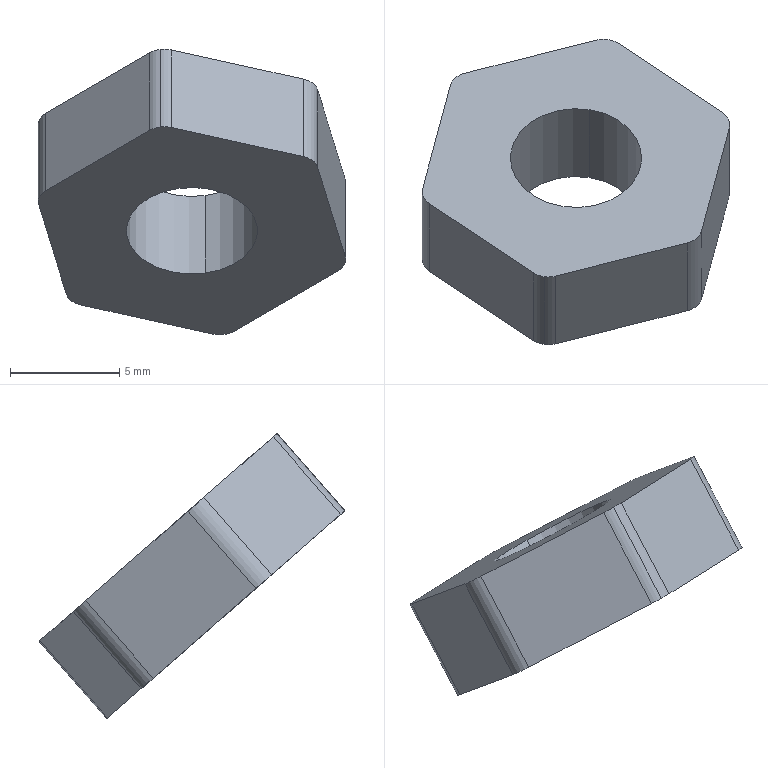Part | STEP file | Fillet 1-12 | 1 solid | 18 faces | box 14.041 x 13.974 x 13.045 mm | volume 553.479 mm3 | cylinder 10 | plane 8 | commonest cylinder face diameters 2 x8 6 x2
STEP:
#1=CARTESIAN_POINT('',(289.281,-940.08,2894.843));
#2=VERTEX_POINT('',#1);
#3=CARTESIAN_POINT('',(288.818,-939.907,2894.691));
#4=VERTEX_POINT('',#3);
#5=CARTESIAN_POINT('',(289.48,-939.342,2894.198));
#6=DIRECTION('',(0.,-0.6579,-0.7531));
#7=DIRECTION('',(0.1984,0.7382,-0.6448));
#8=AXIS2_PLACEMENT_3D('',#5,#6,#7);
#9=CIRCLE('',#8,1.);
#10=EDGE_CURVE('',#2,#4,#9,.T.);
#11=ORIENTED_EDGE('',*,*,#10,.F.);
#12=CARTESIAN_POINT('',(289.281,-936.988,2898.383));
#13=VERTEX_POINT('',#12);
#14=CARTESIAN_POINT('',(289.281,-940.08,2894.843));
#15=DIRECTION('',(0.,0.6579,0.7531));
#16=VECTOR('',#15,1000.);
#17=LINE('',#14,#16);
#18=EDGE_CURVE('',#2,#13,#17,.T.);
#19=ORIENTED_EDGE('',*,*,#18,.T.);
#20=CARTESIAN_POINT('',(288.818,-936.815,2898.231));
#21=VERTEX_POINT('',#20);
#22=CARTESIAN_POINT('',(289.48,-936.25,2897.738));
#23=DIRECTION('',(0.,0.6579,0.7531));
#24=DIRECTION('',(0.1984,0.7382,-0.6448));
#25=AXIS2_PLACEMENT_3D('',#22,#23,#24);
#26=CIRCLE('',#25,1.);
#27=EDGE_CURVE('',#21,#13,#26,.T.);
#28=ORIENTED_EDGE('',*,*,#27,.F.);
#29=CARTESIAN_POINT('',(288.818,-939.907,2894.691));
#30=DIRECTION('',(0.,0.6579,0.7531));
#31=VECTOR('',#30,1000.);
#32=LINE('',#29,#31);
#33=EDGE_CURVE('',#4,#21,#32,.T.);
#34=ORIENTED_EDGE('',*,*,#33,.F.);
#35=EDGE_LOOP('',(#11,#19,#28,#34));
#36=FACE_OUTER_BOUND('',#35,.T.);
#37=CARTESIAN_POINT('',(289.48,-939.342,2894.198));
#38=DIRECTION('',(0.,0.6579,0.7531));
#39=DIRECTION('',(-0.1984,-0.7382,0.6448));
#40=AXIS2_PLACEMENT_3D('',#37,#38,#39);
#41=CYLINDRICAL_SURFACE('',#40,1.);
#42=ADVANCED_FACE('',(#36),#41,.T.);
#43=CARTESIAN_POINT('',(292.198,-929.228,2885.364));
#44=VERTEX_POINT('',#43);
#45=CARTESIAN_POINT('',(292.661,-929.402,2885.515));
#46=VERTEX_POINT('',#45);
#47=CARTESIAN_POINT('',(292.,-929.966,2886.008));
#48=DIRECTION('',(0.,-0.6579,-0.7531));
#49=DIRECTION('',(0.1984,0.7382,-0.6448));
#50=AXIS2_PLACEMENT_3D('',#47,#48,#49);
#51=CIRCLE('',#50,1.);
#52=EDGE_CURVE('',#44,#46,#51,.T.);
#53=ORIENTED_EDGE('',*,*,#52,.F.);
#54=CARTESIAN_POINT('',(292.198,-926.136,2888.903));
#55=VERTEX_POINT('',#54);
#56=CARTESIAN_POINT('',(292.198,-929.228,2885.364));
#57=DIRECTION('',(0.,0.6579,0.7531));
#58=VECTOR('',#57,1000.);
#59=LINE('',#56,#58);
#60=EDGE_CURVE('',#44,#55,#59,.T.);
#61=ORIENTED_EDGE('',*,*,#60,.T.);
#62=CARTESIAN_POINT('',(292.661,-926.31,2889.055));
#63=VERTEX_POINT('',#62);
#64=CARTESIAN_POINT('',(292.,-926.874,2889.548));
#65=DIRECTION('',(0.,0.6579,0.7531));
#66=DIRECTION('',(0.1984,0.7382,-0.6448));
#67=AXIS2_PLACEMENT_3D('',#64,#65,#66);
#68=CIRCLE('',#67,1.);
#69=EDGE_CURVE('',#63,#55,#68,.T.);
#70=ORIENTED_EDGE('',*,*,#69,.F.);
#71=CARTESIAN_POINT('',(292.661,-929.402,2885.515));
#72=DIRECTION('',(0.,0.6579,0.7531));
#73=VECTOR('',#72,1000.);
#74=LINE('',#71,#73);
#75=EDGE_CURVE('',#46,#63,#74,.T.);
#76=ORIENTED_EDGE('',*,*,#75,.F.);
#77=EDGE_LOOP('',(#53,#61,#70,#76));
#78=FACE_OUTER_BOUND('',#77,.T.);
#79=CARTESIAN_POINT('',(292.,-929.966,2886.008));
#80=DIRECTION('',(0.,0.6579,0.7531));
#81=DIRECTION('',(-0.1984,-0.7382,0.6448));
#82=AXIS2_PLACEMENT_3D('',#79,#80,#81);
#83=CYLINDRICAL_SURFACE('',#82,1.);
#84=ADVANCED_FACE('',(#78),#83,.T.);
#85=CARTESIAN_POINT('',(290.144,-936.869,2892.038));
#86=VERTEX_POINT('',#85);
#87=CARTESIAN_POINT('',(291.335,-932.44,2888.169));
#88=VERTEX_POINT('',#87);
#89=CARTESIAN_POINT('',(290.74,-934.654,2890.103));
#90=DIRECTION('',(0.,0.6579,0.7531));
#91=DIRECTION('',(0.1984,0.7382,-0.6448));
#92=AXIS2_PLACEMENT_3D('',#89,#90,#91);
#93=CIRCLE('',#92,3.);
#94=EDGE_CURVE('',#86,#88,#93,.T.);
#95=ORIENTED_EDGE('',*,*,#94,.F.);
#96=CARTESIAN_POINT('',(290.144,-933.777,2895.578));
#97=VERTEX_POINT('',#96);
#98=CARTESIAN_POINT('',(290.144,-938.711,2889.929));
#99=DIRECTION('',(0.,0.6579,0.7531));
#100=VECTOR('',#99,1000.);
#101=LINE('',#98,#100);
#102=EDGE_CURVE('',#86,#97,#101,.T.);
#103=ORIENTED_EDGE('',*,*,#102,.T.);
#104=CARTESIAN_POINT('',(291.335,-929.348,2891.709));
#105=VERTEX_POINT('',#104);
#106=CARTESIAN_POINT('',(290.74,-931.562,2893.643));
#107=DIRECTION('',(0.,0.6579,0.7531));
#108=DIRECTION('',(0.1984,0.7382,-0.6448));
#109=AXIS2_PLACEMENT_3D('',#106,#107,#108);
#110=CIRCLE('',#109,3.);
#111=EDGE_CURVE('',#97,#105,#110,.T.);
#112=ORIENTED_EDGE('',*,*,#111,.T.);
#113=CARTESIAN_POINT('',(291.335,-934.282,2886.06));
#114=DIRECTION('',(0.,0.6579,0.7531));
#115=VECTOR('',#114,1000.);
#116=LINE('',#113,#115);
#117=EDGE_CURVE('',#88,#105,#116,.T.);
#118=ORIENTED_EDGE('',*,*,#117,.F.);
#119=EDGE_LOOP('',(#95,#103,#112,#118));
#120=FACE_OUTER_BOUND('',#119,.T.);
#121=CARTESIAN_POINT('',(290.74,-936.496,2887.995));
#122=DIRECTION('',(0.,0.6579,0.7531));
#123=DIRECTION('',(-0.1984,-0.7382,0.6448));
#124=AXIS2_PLACEMENT_3D('',#121,#122,#123);
#125=CYLINDRICAL_SURFACE('',#124,3.);
#126=ADVANCED_FACE('',(#120),#125,.F.);
#127=CARTESIAN_POINT('',(297.422,-932.568,2888.281));
#128=VERTEX_POINT('',#127);
#129=CARTESIAN_POINT('',(297.855,-932.855,2888.532));
#130=DIRECTION('',(-0.7496,0.4985,-0.4354));
#131=VECTOR('',#130,1000.);
#132=LINE('',#129,#131);
#133=EDGE_CURVE('',#128,#46,#132,.T.);
#134=ORIENTED_EDGE('',*,*,#133,.T.);
#135=ORIENTED_EDGE('',*,*,#75,.T.);
#136=CARTESIAN_POINT('',(297.422,-929.476,2891.82));
#137=VERTEX_POINT('',#136);
#138=CARTESIAN_POINT('',(297.855,-929.763,2892.072));
#139=DIRECTION('',(-0.7496,0.4985,-0.4354));
#140=VECTOR('',#139,1000.);
#141=LINE('',#138,#140);
#142=EDGE_CURVE('',#137,#63,#141,.T.);
#143=ORIENTED_EDGE('',*,*,#142,.F.);
#144=CARTESIAN_POINT('',(297.422,-932.568,2888.281));
#145=DIRECTION('',(0.,-0.6579,-0.7531));
#146=VECTOR('',#145,1000.);
#147=LINE('',#144,#146);
#148=EDGE_CURVE('',#137,#128,#147,.T.);
#149=ORIENTED_EDGE('',*,*,#148,.T.);
#150=EDGE_LOOP('',(#134,#135,#143,#149));
#151=FACE_OUTER_BOUND('',#150,.T.);
#152=CARTESIAN_POINT('',(297.855,-932.855,2888.532));
#153=DIRECTION('',(0.6619,0.5646,-0.4931));
#154=DIRECTION('',(0.7496,-0.4985,0.4354));
#155=AXIS2_PLACEMENT_3D('',#152,#153,#154);
#156=PLANE('',#155);
#157=ADVANCED_FACE('',(#151),#156,.T.);
#158=CARTESIAN_POINT('',(296.48,-937.97,2892.999));
#159=VERTEX_POINT('',#158);
#160=CARTESIAN_POINT('',(297.74,-933.282,2888.904));
#161=VERTEX_POINT('',#160);
#162=CARTESIAN_POINT('',(296.366,-938.396,2893.372));
#163=DIRECTION('',(0.1984,0.7382,-0.6448));
#164=VECTOR('',#163,1000.);
#165=LINE('',#162,#164);
#166=EDGE_CURVE('',#159,#161,#165,.T.);
#167=ORIENTED_EDGE('',*,*,#166,.T.);
#168=CARTESIAN_POINT('',(297.74,-930.19,2892.444));
#169=VERTEX_POINT('',#168);
#170=CARTESIAN_POINT('',(297.74,-933.282,2888.904));
#171=DIRECTION('',(0.,0.6579,0.7531));
#172=VECTOR('',#171,1000.);
#173=LINE('',#170,#172);
#174=EDGE_CURVE('',#161,#169,#173,.T.);
#175=ORIENTED_EDGE('',*,*,#174,.T.);
#176=CARTESIAN_POINT('',(296.48,-934.878,2896.539));
#177=VERTEX_POINT('',#176);
#178=CARTESIAN_POINT('',(296.366,-935.304,2896.911));
#179=DIRECTION('',(0.1984,0.7382,-0.6448));
#180=VECTOR('',#179,1000.);
#181=LINE('',#178,#180);
#182=EDGE_CURVE('',#177,#169,#181,.T.);
#183=ORIENTED_EDGE('',*,*,#182,.F.);
#184=CARTESIAN_POINT('',(296.48,-937.97,2892.999));
#185=DIRECTION('',(0.,-0.6579,-0.7531));
#186=VECTOR('',#185,1000.);
#187=LINE('',#184,#186);
#188=EDGE_CURVE('',#177,#159,#187,.T.);
#189=ORIENTED_EDGE('',*,*,#188,.T.);
#190=EDGE_LOOP('',(#167,#175,#183,#189));
#191=FACE_OUTER_BOUND('',#190,.T.);
#192=CARTESIAN_POINT('',(296.366,-938.396,2893.372));
#193=DIRECTION('',(0.9801,-0.1494,0.1305));
#194=DIRECTION('',(-0.1984,-0.7382,0.6448));
#195=AXIS2_PLACEMENT_3D('',#192,#193,#194);
#196=PLANE('',#195);
#197=ADVANCED_FACE('',(#191),#196,.T.);
#198=CARTESIAN_POINT('',(289.798,-940.056,2894.822));
#199=VERTEX_POINT('',#198);
#200=CARTESIAN_POINT('',(295.818,-938.534,2893.492));
#201=VERTEX_POINT('',#200);
#202=CARTESIAN_POINT('',(289.25,-940.195,2894.943));
#203=DIRECTION('',(0.948,0.2397,-0.2094));
#204=VECTOR('',#203,1000.);
#205=LINE('',#202,#204);
#206=EDGE_CURVE('',#199,#201,#205,.T.);
#207=ORIENTED_EDGE('',*,*,#206,.T.);
#208=CARTESIAN_POINT('',(295.818,-935.442,2897.032));
#209=VERTEX_POINT('',#208);
#210=CARTESIAN_POINT('',(295.818,-938.534,2893.492));
#211=DIRECTION('',(0.,0.6579,0.7531));
#212=VECTOR('',#211,1000.);
#213=LINE('',#210,#212);
#214=EDGE_CURVE('',#201,#209,#213,.T.);
#215=ORIENTED_EDGE('',*,*,#214,.T.);
#216=CARTESIAN_POINT('',(289.798,-936.964,2898.362));
#217=VERTEX_POINT('',#216);
#218=CARTESIAN_POINT('',(289.25,-937.103,2898.483));
#219=DIRECTION('',(0.948,0.2397,-0.2094));
#220=VECTOR('',#219,1000.);
#221=LINE('',#218,#220);
#222=EDGE_CURVE('',#217,#209,#221,.T.);
#223=ORIENTED_EDGE('',*,*,#222,.F.);
#224=CARTESIAN_POINT('',(289.798,-940.056,2894.822));
#225=DIRECTION('',(0.,-0.6579,-0.7531));
#226=VECTOR('',#225,1000.);
#227=LINE('',#224,#226);
#228=EDGE_CURVE('',#217,#199,#227,.T.);
#229=ORIENTED_EDGE('',*,*,#228,.T.);
#230=EDGE_LOOP('',(#207,#215,#223,#229));
#231=FACE_OUTER_BOUND('',#230,.T.);
#232=CARTESIAN_POINT('',(289.25,-940.195,2894.943));
#233=DIRECTION('',(0.3182,-0.714,0.6237));
#234=DIRECTION('',(-0.948,-0.2397,0.2094));
#235=AXIS2_PLACEMENT_3D('',#232,#233,#234);
#236=PLANE('',#235);
#237=ADVANCED_FACE('',(#231),#236,.T.);
#238=CARTESIAN_POINT('',(284.057,-933.649,2895.466));
#239=VERTEX_POINT('',#238);
#240=CARTESIAN_POINT('',(283.624,-933.361,2895.214));
#241=DIRECTION('',(0.7496,-0.4985,0.4354));
#242=VECTOR('',#241,1000.);
#243=LINE('',#240,#242);
#244=EDGE_CURVE('',#239,#21,#243,.T.);
#245=ORIENTED_EDGE('',*,*,#244,.F.);
#246=CARTESIAN_POINT('',(284.057,-936.741,2891.926));
#247=VERTEX_POINT('',#246);
#248=CARTESIAN_POINT('',(284.057,-936.741,2891.926));
#249=DIRECTION('',(0.,-0.6579,-0.7531));
#250=VECTOR('',#249,1000.);
#251=LINE('',#248,#250);
#252=EDGE_CURVE('',#239,#247,#251,.T.);
#253=ORIENTED_EDGE('',*,*,#252,.T.);
#254=CARTESIAN_POINT('',(283.624,-936.453,2891.675));
#255=DIRECTION('',(0.7496,-0.4985,0.4354));
#256=VECTOR('',#255,1000.);
#257=LINE('',#254,#256);
#258=EDGE_CURVE('',#247,#4,#257,.T.);
#259=ORIENTED_EDGE('',*,*,#258,.T.);
#260=ORIENTED_EDGE('',*,*,#33,.T.);
#261=EDGE_LOOP('',(#245,#253,#259,#260));
#262=FACE_OUTER_BOUND('',#261,.T.);
#263=CARTESIAN_POINT('',(283.624,-936.453,2891.675));
#264=DIRECTION('',(-0.6619,-0.5646,0.4931));
#265=DIRECTION('',(-0.7496,0.4985,-0.4354));
#266=AXIS2_PLACEMENT_3D('',#263,#264,#265);
#267=PLANE('',#266);
#268=ADVANCED_FACE('',(#262),#267,.T.);
#269=CARTESIAN_POINT('',(284.999,-931.339,2887.208));
#270=VERTEX_POINT('',#269);
#271=CARTESIAN_POINT('',(283.739,-936.027,2891.302));
#272=VERTEX_POINT('',#271);
#273=CARTESIAN_POINT('',(285.113,-930.913,2886.835));
#274=DIRECTION('',(-0.1984,-0.7382,0.6448));
#275=VECTOR('',#274,1000.);
#276=LINE('',#273,#275);
#277=EDGE_CURVE('',#270,#272,#276,.T.);
#278=ORIENTED_EDGE('',*,*,#277,.T.);
#279=CARTESIAN_POINT('',(283.739,-932.935,2894.842));
#280=VERTEX_POINT('',#279);
#281=CARTESIAN_POINT('',(283.739,-936.027,2891.302));
#282=DIRECTION('',(0.,0.6579,0.7531));
#283=VECTOR('',#282,1000.);
#284=LINE('',#281,#283);
#285=EDGE_CURVE('',#272,#280,#284,.T.);
#286=ORIENTED_EDGE('',*,*,#285,.T.);
#287=CARTESIAN_POINT('',(284.999,-928.247,2890.747));
#288=VERTEX_POINT('',#287);
#289=CARTESIAN_POINT('',(285.113,-927.821,2890.375));
#290=DIRECTION('',(-0.1984,-0.7382,0.6448));
#291=VECTOR('',#290,1000.);
#292=LINE('',#289,#291);
#293=EDGE_CURVE('',#288,#280,#292,.T.);
#294=ORIENTED_EDGE('',*,*,#293,.F.);
#295=CARTESIAN_POINT('',(284.999,-931.339,2887.208));
#296=DIRECTION('',(0.,-0.6579,-0.7531));
#297=VECTOR('',#296,1000.);
#298=LINE('',#295,#297);
#299=EDGE_CURVE('',#288,#270,#298,.T.);
#300=ORIENTED_EDGE('',*,*,#299,.T.);
#301=EDGE_LOOP('',(#278,#286,#294,#300));
#302=FACE_OUTER_BOUND('',#301,.T.);
#303=CARTESIAN_POINT('',(285.113,-930.913,2886.835));
#304=DIRECTION('',(-0.9801,0.1494,-0.1305));
#305=DIRECTION('',(0.1984,0.7382,-0.6448));
#306=AXIS2_PLACEMENT_3D('',#303,#304,#305);
#307=PLANE('',#306);
#308=ADVANCED_FACE('',(#302),#307,.T.);
#309=CARTESIAN_POINT('',(291.681,-929.252,2885.385));
#310=VERTEX_POINT('',#309);
#311=CARTESIAN_POINT('',(285.661,-930.774,2886.714));
#312=VERTEX_POINT('',#311);
#313=CARTESIAN_POINT('',(292.229,-929.114,2885.264));
#314=DIRECTION('',(-0.948,-0.2397,0.2094));
#315=VECTOR('',#314,1000.);
#316=LINE('',#313,#315);
#317=EDGE_CURVE('',#310,#312,#316,.T.);
#318=ORIENTED_EDGE('',*,*,#317,.T.);
#319=CARTESIAN_POINT('',(285.661,-927.682,2890.254));
#320=VERTEX_POINT('',#319);
#321=CARTESIAN_POINT('',(285.661,-930.774,2886.714));
#322=DIRECTION('',(0.,0.6579,0.7531));
#323=VECTOR('',#322,1000.);
#324=LINE('',#321,#323);
#325=EDGE_CURVE('',#312,#320,#324,.T.);
#326=ORIENTED_EDGE('',*,*,#325,.T.);
#327=CARTESIAN_POINT('',(291.681,-926.16,2888.925));
#328=VERTEX_POINT('',#327);
#329=CARTESIAN_POINT('',(292.229,-926.022,2888.804));
#330=DIRECTION('',(-0.948,-0.2397,0.2094));
#331=VECTOR('',#330,1000.);
#332=LINE('',#329,#331);
#333=EDGE_CURVE('',#328,#320,#332,.T.);
#334=ORIENTED_EDGE('',*,*,#333,.F.);
#335=CARTESIAN_POINT('',(291.681,-929.252,2885.385));
#336=DIRECTION('',(0.,-0.6579,-0.7531));
#337=VECTOR('',#336,1000.);
#338=LINE('',#335,#337);
#339=EDGE_CURVE('',#328,#310,#338,.T.);
#340=ORIENTED_EDGE('',*,*,#339,.T.);
#341=EDGE_LOOP('',(#318,#326,#334,#340));
#342=FACE_OUTER_BOUND('',#341,.T.);
#343=CARTESIAN_POINT('',(292.229,-929.114,2885.264));
#344=DIRECTION('',(-0.3182,0.714,-0.6237));
#345=DIRECTION('',(0.948,0.2397,-0.2094));
#346=AXIS2_PLACEMENT_3D('',#343,#344,#345);
#347=PLANE('',#346);
#348=ADVANCED_FACE('',(#342),#347,.T.);
#349=CARTESIAN_POINT('',(290.74,-934.654,2890.103));
#350=DIRECTION('',(0.,0.6579,0.7531));
#351=DIRECTION('',(0.1984,0.7382,-0.6448));
#352=AXIS2_PLACEMENT_3D('',#349,#350,#351);
#353=CIRCLE('',#352,3.);
#354=EDGE_CURVE('',#88,#86,#353,.T.);
#355=ORIENTED_EDGE('',*,*,#354,.T.);
#356=ORIENTED_EDGE('',*,*,#94,.T.);
#357=EDGE_LOOP('',(#355,#356));
#358=FACE_BOUND('',#357,.T.);
#359=ORIENTED_EDGE('',*,*,#258,.F.);
#360=CARTESIAN_POINT('',(284.719,-936.176,2891.433));
#361=DIRECTION('',(0.,-0.6579,-0.7531));
#362=DIRECTION('',(0.1984,0.7382,-0.6448));
#363=AXIS2_PLACEMENT_3D('',#360,#361,#362);
#364=CIRCLE('',#363,1.);
#365=EDGE_CURVE('',#247,#272,#364,.T.);
#366=ORIENTED_EDGE('',*,*,#365,.T.);
#367=ORIENTED_EDGE('',*,*,#277,.F.);
#368=CARTESIAN_POINT('',(285.979,-931.488,2887.338));
#369=DIRECTION('',(0.,-0.6579,-0.7531));
#370=DIRECTION('',(0.1984,0.7382,-0.6448));
#371=AXIS2_PLACEMENT_3D('',#368,#369,#370);
#372=CIRCLE('',#371,1.);
#373=EDGE_CURVE('',#270,#312,#372,.T.);
#374=ORIENTED_EDGE('',*,*,#373,.T.);
#375=ORIENTED_EDGE('',*,*,#317,.F.);
#376=CARTESIAN_POINT('',(292.,-929.966,2886.008));
#377=DIRECTION('',(0.,-0.6579,-0.7531));
#378=DIRECTION('',(0.1984,0.7382,-0.6448));
#379=AXIS2_PLACEMENT_3D('',#376,#377,#378);
#380=CIRCLE('',#379,1.);
#381=EDGE_CURVE('',#310,#44,#380,.T.);
#382=ORIENTED_EDGE('',*,*,#381,.T.);
#383=ORIENTED_EDGE('',*,*,#52,.T.);
#384=ORIENTED_EDGE('',*,*,#133,.F.);
#385=CARTESIAN_POINT('',(296.76,-933.132,2888.774));
#386=DIRECTION('',(0.,-0.6579,-0.7531));
#387=DIRECTION('',(0.1984,0.7382,-0.6448));
#388=AXIS2_PLACEMENT_3D('',#385,#386,#387);
#389=CIRCLE('',#388,1.);
#390=EDGE_CURVE('',#128,#161,#389,.T.);
#391=ORIENTED_EDGE('',*,*,#390,.T.);
#392=ORIENTED_EDGE('',*,*,#166,.F.);
#393=CARTESIAN_POINT('',(295.5,-937.82,2892.869));
#394=DIRECTION('',(0.,-0.6579,-0.7531));
#395=DIRECTION('',(0.1984,0.7382,-0.6448));
#396=AXIS2_PLACEMENT_3D('',#393,#394,#395);
#397=CIRCLE('',#396,1.);
#398=EDGE_CURVE('',#159,#201,#397,.T.);
#399=ORIENTED_EDGE('',*,*,#398,.T.);
#400=ORIENTED_EDGE('',*,*,#206,.F.);
#401=CARTESIAN_POINT('',(289.48,-939.342,2894.198));
#402=DIRECTION('',(0.,-0.6579,-0.7531));
#403=DIRECTION('',(0.1984,0.7382,-0.6448));
#404=AXIS2_PLACEMENT_3D('',#401,#402,#403);
#405=CIRCLE('',#404,1.);
#406=EDGE_CURVE('',#199,#2,#405,.T.);
#407=ORIENTED_EDGE('',*,*,#406,.T.);
#408=ORIENTED_EDGE('',*,*,#10,.T.);
#409=EDGE_LOOP('',(#359,#366,#367,#374,#375,#382,#383,#384,#391,#392,#399,#400,#407,#408));
#410=FACE_OUTER_BOUND('',#409,.T.);
#411=CARTESIAN_POINT('',(291.01,-933.648,2889.225));
#412=DIRECTION('',(0.,0.6579,0.7531));
#413=DIRECTION('',(-0.1984,-0.7382,0.6448));
#414=AXIS2_PLACEMENT_3D('',#411,#412,#413);
#415=PLANE('',#414);
#416=ADVANCED_FACE('',(#358,#410),#415,.F.);
#417=CARTESIAN_POINT('',(290.74,-931.562,2893.643));
#418=DIRECTION('',(0.,0.6579,0.7531));
#419=DIRECTION('',(0.1984,0.7382,-0.6448));
#420=AXIS2_PLACEMENT_3D('',#417,#418,#419);
#421=CIRCLE('',#420,3.);
#422=EDGE_CURVE('',#105,#97,#421,.T.);
#423=ORIENTED_EDGE('',*,*,#422,.F.);
#424=ORIENTED_EDGE('',*,*,#111,.F.);
#425=EDGE_LOOP('',(#423,#424));
#426=FACE_BOUND('',#425,.T.);
#427=ORIENTED_EDGE('',*,*,#293,.T.);
#428=CARTESIAN_POINT('',(284.719,-933.084,2894.973));
#429=DIRECTION('',(0.,0.6579,0.7531));
#430=DIRECTION('',(0.1984,0.7382,-0.6448));
#431=AXIS2_PLACEMENT_3D('',#428,#429,#430);
#432=CIRCLE('',#431,1.);
#433=EDGE_CURVE('',#280,#239,#432,.T.);
#434=ORIENTED_EDGE('',*,*,#433,.T.);
#435=ORIENTED_EDGE('',*,*,#244,.T.);
#436=ORIENTED_EDGE('',*,*,#27,.T.);
#437=CARTESIAN_POINT('',(289.48,-936.25,2897.738));
#438=DIRECTION('',(0.,0.6579,0.7531));
#439=DIRECTION('',(0.1984,0.7382,-0.6448));
#440=AXIS2_PLACEMENT_3D('',#437,#438,#439);
#441=CIRCLE('',#440,1.);
#442=EDGE_CURVE('',#13,#217,#441,.T.);
#443=ORIENTED_EDGE('',*,*,#442,.T.);
#444=ORIENTED_EDGE('',*,*,#222,.T.);
#445=CARTESIAN_POINT('',(295.5,-934.728,2896.408));
#446=DIRECTION('',(0.,0.6579,0.7531));
#447=DIRECTION('',(0.1984,0.7382,-0.6448));
#448=AXIS2_PLACEMENT_3D('',#445,#446,#447);
#449=CIRCLE('',#448,1.);
#450=EDGE_CURVE('',#209,#177,#449,.T.);
#451=ORIENTED_EDGE('',*,*,#450,.T.);
#452=ORIENTED_EDGE('',*,*,#182,.T.);
#453=CARTESIAN_POINT('',(296.76,-930.04,2892.314));
#454=DIRECTION('',(0.,0.6579,0.7531));
#455=DIRECTION('',(0.1984,0.7382,-0.6448));
#456=AXIS2_PLACEMENT_3D('',#453,#454,#455);
#457=CIRCLE('',#456,1.);
#458=EDGE_CURVE('',#169,#137,#457,.T.);
#459=ORIENTED_EDGE('',*,*,#458,.T.);
#460=ORIENTED_EDGE('',*,*,#142,.T.);
#461=ORIENTED_EDGE('',*,*,#69,.T.);
#462=CARTESIAN_POINT('',(292.,-926.874,2889.548));
#463=DIRECTION('',(0.,0.6579,0.7531));
#464=DIRECTION('',(0.1984,0.7382,-0.6448));
#465=AXIS2_PLACEMENT_3D('',#462,#463,#464);
#466=CIRCLE('',#465,1.);
#467=EDGE_CURVE('',#55,#328,#466,.T.);
#468=ORIENTED_EDGE('',*,*,#467,.T.);
#469=ORIENTED_EDGE('',*,*,#333,.T.);
#470=CARTESIAN_POINT('',(285.979,-928.396,2890.878));
#471=DIRECTION('',(0.,0.6579,0.7531));
#472=DIRECTION('',(0.1984,0.7382,-0.6448));
#473=AXIS2_PLACEMENT_3D('',#470,#471,#472);
#474=CIRCLE('',#473,1.);
#475=EDGE_CURVE('',#320,#288,#474,.T.);
#476=ORIENTED_EDGE('',*,*,#475,.T.);
#477=EDGE_LOOP('',(#427,#434,#435,#436,#443,#444,#451,#452,#459,#460,#461,#468,#469,#476));
#478=FACE_OUTER_BOUND('',#477,.T.);
#479=CARTESIAN_POINT('',(291.01,-930.557,2892.765));
#480=DIRECTION('',(0.,0.6579,0.7531));
#481=DIRECTION('',(-0.1984,-0.7382,0.6448));
#482=AXIS2_PLACEMENT_3D('',#479,#480,#481);
#483=PLANE('',#482);
#484=ADVANCED_FACE('',(#426,#478),#483,.T.);
#485=ORIENTED_EDGE('',*,*,#102,.F.);
#486=ORIENTED_EDGE('',*,*,#354,.F.);
#487=ORIENTED_EDGE('',*,*,#117,.T.);
#488=ORIENTED_EDGE('',*,*,#422,.T.);
#489=EDGE_LOOP('',(#485,#486,#487,#488));
#490=FACE_OUTER_BOUND('',#489,.T.);
#491=CARTESIAN_POINT('',(290.74,-936.496,2887.995));
#492=DIRECTION('',(0.,0.6579,0.7531));
#493=DIRECTION('',(-0.1984,-0.7382,0.6448));
#494=AXIS2_PLACEMENT_3D('',#491,#492,#493);
#495=CYLINDRICAL_SURFACE('',#494,3.);
#496=ADVANCED_FACE('',(#490),#495,.F.);
#497=ORIENTED_EDGE('',*,*,#365,.F.);
#498=ORIENTED_EDGE('',*,*,#252,.F.);
#499=ORIENTED_EDGE('',*,*,#433,.F.);
#500=ORIENTED_EDGE('',*,*,#285,.F.);
#501=EDGE_LOOP('',(#497,#498,#499,#500));
#502=FACE_OUTER_BOUND('',#501,.T.);
#503=CARTESIAN_POINT('',(284.719,-936.176,2891.433));
#504=DIRECTION('',(0.,0.6579,0.7531));
#505=DIRECTION('',(-0.1984,-0.7382,0.6448));
#506=AXIS2_PLACEMENT_3D('',#503,#504,#505);
#507=CYLINDRICAL_SURFACE('',#506,1.);
#508=ADVANCED_FACE('',(#502),#507,.T.);
#509=ORIENTED_EDGE('',*,*,#373,.F.);
#510=ORIENTED_EDGE('',*,*,#299,.F.);
#511=ORIENTED_EDGE('',*,*,#475,.F.);
#512=ORIENTED_EDGE('',*,*,#325,.F.);
#513=EDGE_LOOP('',(#509,#510,#511,#512));
#514=FACE_OUTER_BOUND('',#513,.T.);
#515=CARTESIAN_POINT('',(285.979,-931.488,2887.338));
#516=DIRECTION('',(0.,0.6579,0.7531));
#517=DIRECTION('',(-0.1984,-0.7382,0.6448));
#518=AXIS2_PLACEMENT_3D('',#515,#516,#517);
#519=CYLINDRICAL_SURFACE('',#518,1.);
#520=ADVANCED_FACE('',(#514),#519,.T.);
#521=ORIENTED_EDGE('',*,*,#60,.F.);
#522=ORIENTED_EDGE('',*,*,#381,.F.);
#523=ORIENTED_EDGE('',*,*,#339,.F.);
#524=ORIENTED_EDGE('',*,*,#467,.F.);
#525=EDGE_LOOP('',(#521,#522,#523,#524));
#526=FACE_OUTER_BOUND('',#525,.T.);
#527=CARTESIAN_POINT('',(292.,-929.966,2886.008));
#528=DIRECTION('',(0.,0.6579,0.7531));
#529=DIRECTION('',(-0.1984,-0.7382,0.6448));
#530=AXIS2_PLACEMENT_3D('',#527,#528,#529);
#531=CYLINDRICAL_SURFACE('',#530,1.);
#532=ADVANCED_FACE('',(#526),#531,.T.);
#533=ORIENTED_EDGE('',*,*,#390,.F.);
#534=ORIENTED_EDGE('',*,*,#148,.F.);
#535=ORIENTED_EDGE('',*,*,#458,.F.);
#536=ORIENTED_EDGE('',*,*,#174,.F.);
#537=EDGE_LOOP('',(#533,#534,#535,#536));
#538=FACE_OUTER_BOUND('',#537,.T.);
#539=CARTESIAN_POINT('',(296.76,-933.132,2888.774));
#540=DIRECTION('',(0.,0.6579,0.7531));
#541=DIRECTION('',(-0.1984,-0.7382,0.6448));
#542=AXIS2_PLACEMENT_3D('',#539,#540,#541);
#543=CYLINDRICAL_SURFACE('',#542,1.);
#544=ADVANCED_FACE('',(#538),#543,.T.);
#545=ORIENTED_EDGE('',*,*,#398,.F.);
#546=ORIENTED_EDGE('',*,*,#188,.F.);
#547=ORIENTED_EDGE('',*,*,#450,.F.);
#548=ORIENTED_EDGE('',*,*,#214,.F.);
#549=EDGE_LOOP('',(#545,#546,#547,#548));
#550=FACE_OUTER_BOUND('',#549,.T.);
#551=CARTESIAN_POINT('',(295.5,-937.82,2892.869));
#552=DIRECTION('',(0.,0.6579,0.7531));
#553=DIRECTION('',(-0.1984,-0.7382,0.6448));
#554=AXIS2_PLACEMENT_3D('',#551,#552,#553);
#555=CYLINDRICAL_SURFACE('',#554,1.);
#556=ADVANCED_FACE('',(#550),#555,.T.);
#557=ORIENTED_EDGE('',*,*,#18,.F.);
#558=ORIENTED_EDGE('',*,*,#406,.F.);
#559=ORIENTED_EDGE('',*,*,#228,.F.);
#560=ORIENTED_EDGE('',*,*,#442,.F.);
#561=EDGE_LOOP('',(#557,#558,#559,#560));
#562=FACE_OUTER_BOUND('',#561,.T.);
#563=CARTESIAN_POINT('',(289.48,-939.342,2894.198));
#564=DIRECTION('',(0.,0.6579,0.7531));
#565=DIRECTION('',(-0.1984,-0.7382,0.6448));
#566=AXIS2_PLACEMENT_3D('',#563,#564,#565);
#567=CYLINDRICAL_SURFACE('',#566,1.);
#568=ADVANCED_FACE('',(#562),#567,.T.);
#569=CLOSED_SHELL('',(#42,#84,#126,#157,#197,#237,#268,#308,#348,#416,#484,#496,#508,#520,#532,#544,#556,#568));
#570=MANIFOLD_SOLID_BREP('',#569);
#571=CARTESIAN_POINT('',(0.,0.,0.));
#572=DIRECTION('',(0.,0.,1.));
#573=DIRECTION('',(1.,0.,0.));
#574=AXIS2_PLACEMENT_3D('',#571,#572,#573);
#575=(LENGTH_UNIT()NAMED_UNIT(*)SI_UNIT(.MILLI.,.METRE.));
#576=UNCERTAINTY_MEASURE_WITH_UNIT(LENGTH_MEASURE(0.00001),#575,'','');
#577=(NAMED_UNIT(*)PLANE_ANGLE_UNIT()SI_UNIT($,.RADIAN.));
#578=(NAMED_UNIT(*)SI_UNIT($,.STERADIAN.)SOLID_ANGLE_UNIT());
#579=(GEOMETRIC_REPRESENTATION_CONTEXT(3)GLOBAL_UNCERTAINTY_ASSIGNED_CONTEXT((#576))GLOBAL_UNIT_ASSIGNED_CONTEXT((#575,#577,#578))REPRESENTATION_CONTEXT('',''));
#580=ADVANCED_BREP_SHAPE_REPRESENTATION('',(#570,#574),#579);